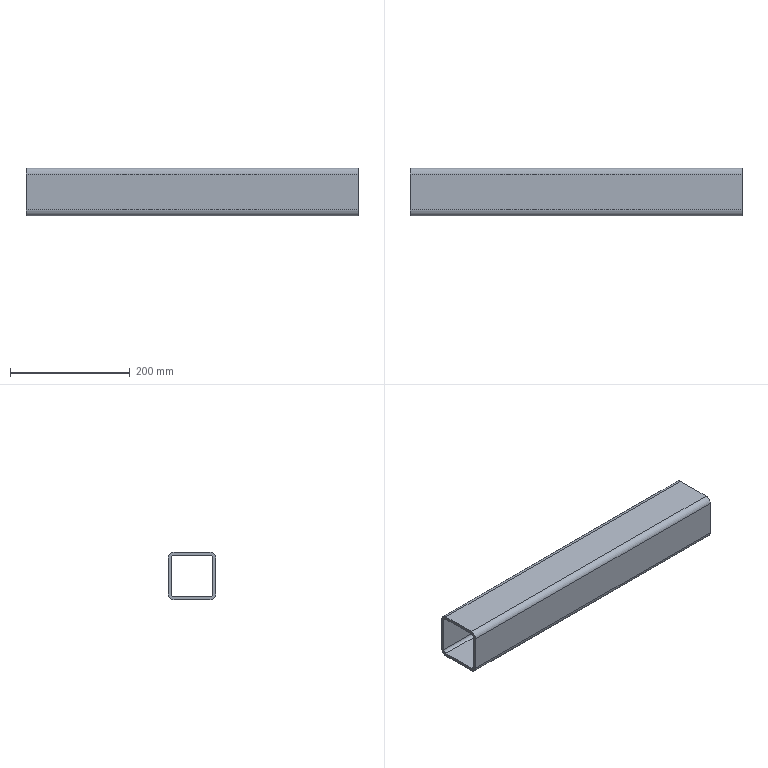Part | SolidWorks | features BaseBody 1 | 1 solid | 18 faces | box 555 x 80 x 80 mm | volume 796769 mm3 | plane 10 | cylinder 8 | commonest cylinder face diameters 10 x4 20 x4
STEP:
#1=CARTESIAN_POINT('',(-277.5,30.,-40.));
#2=VERTEX_POINT('',#1);
#3=CARTESIAN_POINT('',(-277.5,40.,-30.));
#4=VERTEX_POINT('',#3);
#5=CARTESIAN_POINT('',(-277.5,30.,-30.));
#6=DIRECTION('',(1.,0.,0.));
#7=DIRECTION('',(0.,0.,-1.));
#8=AXIS2_PLACEMENT_3D('',#5,#6,#7);
#9=CIRCLE('',#8,10.);
#10=EDGE_CURVE('',#2,#4,#9,.T.);
#11=ORIENTED_EDGE('',*,*,#10,.T.);
#12=CARTESIAN_POINT('',(277.5,40.,-30.));
#13=VERTEX_POINT('',#12);
#14=CARTESIAN_POINT('',(277.5,40.,-30.));
#15=DIRECTION('',(-1.,0.,0.));
#16=VECTOR('',#15,1000.);
#17=LINE('',#14,#16);
#18=EDGE_CURVE('',#13,#4,#17,.T.);
#19=ORIENTED_EDGE('',*,*,#18,.F.);
#20=CARTESIAN_POINT('',(277.5,30.,-40.));
#21=VERTEX_POINT('',#20);
#22=CARTESIAN_POINT('',(277.5,30.,-30.));
#23=DIRECTION('',(1.,0.,0.));
#24=DIRECTION('',(0.,0.,-1.));
#25=AXIS2_PLACEMENT_3D('',#22,#23,#24);
#26=CIRCLE('',#25,10.);
#27=EDGE_CURVE('',#21,#13,#26,.T.);
#28=ORIENTED_EDGE('',*,*,#27,.F.);
#29=CARTESIAN_POINT('',(277.5,30.,-40.));
#30=DIRECTION('',(-1.,0.,0.));
#31=VECTOR('',#30,1000.);
#32=LINE('',#29,#31);
#33=EDGE_CURVE('',#21,#2,#32,.T.);
#34=ORIENTED_EDGE('',*,*,#33,.T.);
#35=EDGE_LOOP('',(#11,#19,#28,#34));
#36=FACE_OUTER_BOUND('',#35,.T.);
#37=CARTESIAN_POINT('',(277.5,30.,-30.));
#38=DIRECTION('',(-1.,0.,0.));
#39=DIRECTION('',(0.,0.,1.));
#40=AXIS2_PLACEMENT_3D('',#37,#38,#39);
#41=CYLINDRICAL_SURFACE('',#40,10.);
#42=ADVANCED_FACE('',(#36),#41,.T.);
#43=CARTESIAN_POINT('',(-277.5,40.,30.));
#44=VERTEX_POINT('',#43);
#45=CARTESIAN_POINT('',(-277.5,40.,-30.));
#46=DIRECTION('',(0.,0.,1.));
#47=VECTOR('',#46,1000.);
#48=LINE('',#45,#47);
#49=EDGE_CURVE('',#4,#44,#48,.T.);
#50=ORIENTED_EDGE('',*,*,#49,.T.);
#51=CARTESIAN_POINT('',(277.5,40.,30.));
#52=VERTEX_POINT('',#51);
#53=CARTESIAN_POINT('',(277.5,40.,30.));
#54=DIRECTION('',(-1.,0.,0.));
#55=VECTOR('',#54,1000.);
#56=LINE('',#53,#55);
#57=EDGE_CURVE('',#52,#44,#56,.T.);
#58=ORIENTED_EDGE('',*,*,#57,.F.);
#59=CARTESIAN_POINT('',(277.5,40.,-30.));
#60=DIRECTION('',(0.,0.,1.));
#61=VECTOR('',#60,1000.);
#62=LINE('',#59,#61);
#63=EDGE_CURVE('',#13,#52,#62,.T.);
#64=ORIENTED_EDGE('',*,*,#63,.F.);
#65=ORIENTED_EDGE('',*,*,#18,.T.);
#66=EDGE_LOOP('',(#50,#58,#64,#65));
#67=FACE_OUTER_BOUND('',#66,.T.);
#68=CARTESIAN_POINT('',(277.5,40.,-30.));
#69=DIRECTION('',(0.,-1.,0.));
#70=DIRECTION('',(0.,0.,-1.));
#71=AXIS2_PLACEMENT_3D('',#68,#69,#70);
#72=PLANE('',#71);
#73=ADVANCED_FACE('',(#67),#72,.F.);
#74=CARTESIAN_POINT('',(-277.5,30.,40.));
#75=VERTEX_POINT('',#74);
#76=CARTESIAN_POINT('',(-277.5,30.,30.));
#77=DIRECTION('',(1.,0.,0.));
#78=DIRECTION('',(0.,0.,-1.));
#79=AXIS2_PLACEMENT_3D('',#76,#77,#78);
#80=CIRCLE('',#79,10.);
#81=EDGE_CURVE('',#44,#75,#80,.T.);
#82=ORIENTED_EDGE('',*,*,#81,.T.);
#83=CARTESIAN_POINT('',(277.5,30.,40.));
#84=VERTEX_POINT('',#83);
#85=CARTESIAN_POINT('',(277.5,30.,40.));
#86=DIRECTION('',(-1.,0.,0.));
#87=VECTOR('',#86,1000.);
#88=LINE('',#85,#87);
#89=EDGE_CURVE('',#84,#75,#88,.T.);
#90=ORIENTED_EDGE('',*,*,#89,.F.);
#91=CARTESIAN_POINT('',(277.5,30.,30.));
#92=DIRECTION('',(1.,0.,0.));
#93=DIRECTION('',(0.,0.,-1.));
#94=AXIS2_PLACEMENT_3D('',#91,#92,#93);
#95=CIRCLE('',#94,10.);
#96=EDGE_CURVE('',#52,#84,#95,.T.);
#97=ORIENTED_EDGE('',*,*,#96,.F.);
#98=ORIENTED_EDGE('',*,*,#57,.T.);
#99=EDGE_LOOP('',(#82,#90,#97,#98));
#100=FACE_OUTER_BOUND('',#99,.T.);
#101=CARTESIAN_POINT('',(277.5,30.,30.));
#102=DIRECTION('',(-1.,0.,0.));
#103=DIRECTION('',(0.,0.,1.));
#104=AXIS2_PLACEMENT_3D('',#101,#102,#103);
#105=CYLINDRICAL_SURFACE('',#104,10.);
#106=ADVANCED_FACE('',(#100),#105,.T.);
#107=CARTESIAN_POINT('',(-277.5,-30.,40.));
#108=VERTEX_POINT('',#107);
#109=CARTESIAN_POINT('',(-277.5,-30.,40.));
#110=DIRECTION('',(0.,-1.,0.));
#111=VECTOR('',#110,1000.);
#112=LINE('',#109,#111);
#113=EDGE_CURVE('',#75,#108,#112,.T.);
#114=ORIENTED_EDGE('',*,*,#113,.T.);
#115=CARTESIAN_POINT('',(277.5,-30.,40.));
#116=VERTEX_POINT('',#115);
#117=CARTESIAN_POINT('',(277.5,-30.,40.));
#118=DIRECTION('',(-1.,0.,0.));
#119=VECTOR('',#118,1000.);
#120=LINE('',#117,#119);
#121=EDGE_CURVE('',#116,#108,#120,.T.);
#122=ORIENTED_EDGE('',*,*,#121,.F.);
#123=CARTESIAN_POINT('',(277.5,-30.,40.));
#124=DIRECTION('',(0.,-1.,0.));
#125=VECTOR('',#124,1000.);
#126=LINE('',#123,#125);
#127=EDGE_CURVE('',#84,#116,#126,.T.);
#128=ORIENTED_EDGE('',*,*,#127,.F.);
#129=ORIENTED_EDGE('',*,*,#89,.T.);
#130=EDGE_LOOP('',(#114,#122,#128,#129));
#131=FACE_OUTER_BOUND('',#130,.T.);
#132=CARTESIAN_POINT('',(277.5,-30.,40.));
#133=DIRECTION('',(0.,0.,-1.));
#134=DIRECTION('',(-1.,0.,0.));
#135=AXIS2_PLACEMENT_3D('',#132,#133,#134);
#136=PLANE('',#135);
#137=ADVANCED_FACE('',(#131),#136,.F.);
#138=CARTESIAN_POINT('',(-277.5,-40.,30.));
#139=VERTEX_POINT('',#138);
#140=CARTESIAN_POINT('',(-277.5,-30.,30.));
#141=DIRECTION('',(1.,0.,0.));
#142=DIRECTION('',(0.,0.,-1.));
#143=AXIS2_PLACEMENT_3D('',#140,#141,#142);
#144=CIRCLE('',#143,10.);
#145=EDGE_CURVE('',#108,#139,#144,.T.);
#146=ORIENTED_EDGE('',*,*,#145,.T.);
#147=CARTESIAN_POINT('',(277.5,-40.,30.));
#148=VERTEX_POINT('',#147);
#149=CARTESIAN_POINT('',(277.5,-40.,30.));
#150=DIRECTION('',(-1.,0.,0.));
#151=VECTOR('',#150,1000.);
#152=LINE('',#149,#151);
#153=EDGE_CURVE('',#148,#139,#152,.T.);
#154=ORIENTED_EDGE('',*,*,#153,.F.);
#155=CARTESIAN_POINT('',(277.5,-30.,30.));
#156=DIRECTION('',(1.,0.,0.));
#157=DIRECTION('',(0.,0.,-1.));
#158=AXIS2_PLACEMENT_3D('',#155,#156,#157);
#159=CIRCLE('',#158,10.);
#160=EDGE_CURVE('',#116,#148,#159,.T.);
#161=ORIENTED_EDGE('',*,*,#160,.F.);
#162=ORIENTED_EDGE('',*,*,#121,.T.);
#163=EDGE_LOOP('',(#146,#154,#161,#162));
#164=FACE_OUTER_BOUND('',#163,.T.);
#165=CARTESIAN_POINT('',(277.5,-30.,30.));
#166=DIRECTION('',(-1.,0.,0.));
#167=DIRECTION('',(0.,0.,1.));
#168=AXIS2_PLACEMENT_3D('',#165,#166,#167);
#169=CYLINDRICAL_SURFACE('',#168,10.);
#170=ADVANCED_FACE('',(#164),#169,.T.);
#171=CARTESIAN_POINT('',(-277.5,-40.,-30.));
#172=VERTEX_POINT('',#171);
#173=CARTESIAN_POINT('',(-277.5,-40.,30.));
#174=DIRECTION('',(0.,0.,-1.));
#175=VECTOR('',#174,1000.);
#176=LINE('',#173,#175);
#177=EDGE_CURVE('',#139,#172,#176,.T.);
#178=ORIENTED_EDGE('',*,*,#177,.T.);
#179=CARTESIAN_POINT('',(277.5,-40.,-30.));
#180=VERTEX_POINT('',#179);
#181=CARTESIAN_POINT('',(277.5,-40.,-30.));
#182=DIRECTION('',(-1.,0.,0.));
#183=VECTOR('',#182,1000.);
#184=LINE('',#181,#183);
#185=EDGE_CURVE('',#180,#172,#184,.T.);
#186=ORIENTED_EDGE('',*,*,#185,.F.);
#187=CARTESIAN_POINT('',(277.5,-40.,30.));
#188=DIRECTION('',(0.,0.,-1.));
#189=VECTOR('',#188,1000.);
#190=LINE('',#187,#189);
#191=EDGE_CURVE('',#148,#180,#190,.T.);
#192=ORIENTED_EDGE('',*,*,#191,.F.);
#193=ORIENTED_EDGE('',*,*,#153,.T.);
#194=EDGE_LOOP('',(#178,#186,#192,#193));
#195=FACE_OUTER_BOUND('',#194,.T.);
#196=CARTESIAN_POINT('',(277.5,-40.,30.));
#197=DIRECTION('',(0.,1.,0.));
#198=DIRECTION('',(0.,0.,1.));
#199=AXIS2_PLACEMENT_3D('',#196,#197,#198);
#200=PLANE('',#199);
#201=ADVANCED_FACE('',(#195),#200,.F.);
#202=CARTESIAN_POINT('',(-277.5,-30.,-40.));
#203=VERTEX_POINT('',#202);
#204=CARTESIAN_POINT('',(-277.5,-30.,-30.));
#205=DIRECTION('',(1.,0.,0.));
#206=DIRECTION('',(0.,0.,-1.));
#207=AXIS2_PLACEMENT_3D('',#204,#205,#206);
#208=CIRCLE('',#207,10.);
#209=EDGE_CURVE('',#172,#203,#208,.T.);
#210=ORIENTED_EDGE('',*,*,#209,.T.);
#211=CARTESIAN_POINT('',(277.5,-30.,-40.));
#212=VERTEX_POINT('',#211);
#213=CARTESIAN_POINT('',(277.5,-30.,-40.));
#214=DIRECTION('',(-1.,0.,0.));
#215=VECTOR('',#214,1000.);
#216=LINE('',#213,#215);
#217=EDGE_CURVE('',#212,#203,#216,.T.);
#218=ORIENTED_EDGE('',*,*,#217,.F.);
#219=CARTESIAN_POINT('',(277.5,-30.,-30.));
#220=DIRECTION('',(1.,0.,0.));
#221=DIRECTION('',(0.,0.,-1.));
#222=AXIS2_PLACEMENT_3D('',#219,#220,#221);
#223=CIRCLE('',#222,10.);
#224=EDGE_CURVE('',#180,#212,#223,.T.);
#225=ORIENTED_EDGE('',*,*,#224,.F.);
#226=ORIENTED_EDGE('',*,*,#185,.T.);
#227=EDGE_LOOP('',(#210,#218,#225,#226));
#228=FACE_OUTER_BOUND('',#227,.T.);
#229=CARTESIAN_POINT('',(277.5,-30.,-30.));
#230=DIRECTION('',(-1.,0.,0.));
#231=DIRECTION('',(0.,0.,1.));
#232=AXIS2_PLACEMENT_3D('',#229,#230,#231);
#233=CYLINDRICAL_SURFACE('',#232,10.);
#234=ADVANCED_FACE('',(#228),#233,.T.);
#235=CARTESIAN_POINT('',(-277.5,35.,30.));
#236=VERTEX_POINT('',#235);
#237=CARTESIAN_POINT('',(-277.5,30.,35.));
#238=VERTEX_POINT('',#237);
#239=CARTESIAN_POINT('',(-277.5,30.,30.));
#240=DIRECTION('',(1.,0.,0.));
#241=DIRECTION('',(0.,0.,-1.));
#242=AXIS2_PLACEMENT_3D('',#239,#240,#241);
#243=CIRCLE('',#242,5.);
#244=EDGE_CURVE('',#236,#238,#243,.T.);
#245=ORIENTED_EDGE('',*,*,#244,.F.);
#246=CARTESIAN_POINT('',(277.5,35.,30.));
#247=VERTEX_POINT('',#246);
#248=CARTESIAN_POINT('',(277.5,35.,30.));
#249=DIRECTION('',(-1.,0.,0.));
#250=VECTOR('',#249,1000.);
#251=LINE('',#248,#250);
#252=EDGE_CURVE('',#247,#236,#251,.T.);
#253=ORIENTED_EDGE('',*,*,#252,.F.);
#254=CARTESIAN_POINT('',(277.5,30.,35.));
#255=VERTEX_POINT('',#254);
#256=CARTESIAN_POINT('',(277.5,30.,30.));
#257=DIRECTION('',(1.,0.,0.));
#258=DIRECTION('',(0.,0.,-1.));
#259=AXIS2_PLACEMENT_3D('',#256,#257,#258);
#260=CIRCLE('',#259,5.);
#261=EDGE_CURVE('',#247,#255,#260,.T.);
#262=ORIENTED_EDGE('',*,*,#261,.T.);
#263=CARTESIAN_POINT('',(277.5,30.,35.));
#264=DIRECTION('',(-1.,0.,0.));
#265=VECTOR('',#264,1000.);
#266=LINE('',#263,#265);
#267=EDGE_CURVE('',#255,#238,#266,.T.);
#268=ORIENTED_EDGE('',*,*,#267,.T.);
#269=EDGE_LOOP('',(#245,#253,#262,#268));
#270=FACE_OUTER_BOUND('',#269,.T.);
#271=CARTESIAN_POINT('',(277.5,30.,30.));
#272=DIRECTION('',(-1.,0.,0.));
#273=DIRECTION('',(0.,0.,1.));
#274=AXIS2_PLACEMENT_3D('',#271,#272,#273);
#275=CYLINDRICAL_SURFACE('',#274,5.);
#276=ADVANCED_FACE('',(#270),#275,.F.);
#277=CARTESIAN_POINT('',(-277.5,35.,-30.));
#278=VERTEX_POINT('',#277);
#279=CARTESIAN_POINT('',(-277.5,35.,-30.));
#280=DIRECTION('',(0.,0.,1.));
#281=VECTOR('',#280,1000.);
#282=LINE('',#279,#281);
#283=EDGE_CURVE('',#278,#236,#282,.T.);
#284=ORIENTED_EDGE('',*,*,#283,.F.);
#285=CARTESIAN_POINT('',(277.5,35.,-30.));
#286=VERTEX_POINT('',#285);
#287=CARTESIAN_POINT('',(277.5,35.,-30.));
#288=DIRECTION('',(-1.,0.,0.));
#289=VECTOR('',#288,1000.);
#290=LINE('',#287,#289);
#291=EDGE_CURVE('',#286,#278,#290,.T.);
#292=ORIENTED_EDGE('',*,*,#291,.F.);
#293=CARTESIAN_POINT('',(277.5,35.,-30.));
#294=DIRECTION('',(0.,0.,1.));
#295=VECTOR('',#294,1000.);
#296=LINE('',#293,#295);
#297=EDGE_CURVE('',#286,#247,#296,.T.);
#298=ORIENTED_EDGE('',*,*,#297,.T.);
#299=ORIENTED_EDGE('',*,*,#252,.T.);
#300=EDGE_LOOP('',(#284,#292,#298,#299));
#301=FACE_OUTER_BOUND('',#300,.T.);
#302=CARTESIAN_POINT('',(277.5,35.,-30.));
#303=DIRECTION('',(0.,-1.,0.));
#304=DIRECTION('',(0.,0.,-1.));
#305=AXIS2_PLACEMENT_3D('',#302,#303,#304);
#306=PLANE('',#305);
#307=ADVANCED_FACE('',(#301),#306,.T.);
#308=CARTESIAN_POINT('',(-277.5,30.,-35.));
#309=VERTEX_POINT('',#308);
#310=CARTESIAN_POINT('',(-277.5,30.,-30.));
#311=DIRECTION('',(1.,0.,0.));
#312=DIRECTION('',(0.,0.,-1.));
#313=AXIS2_PLACEMENT_3D('',#310,#311,#312);
#314=CIRCLE('',#313,5.);
#315=EDGE_CURVE('',#309,#278,#314,.T.);
#316=ORIENTED_EDGE('',*,*,#315,.F.);
#317=CARTESIAN_POINT('',(277.5,30.,-35.));
#318=VERTEX_POINT('',#317);
#319=CARTESIAN_POINT('',(277.5,30.,-35.));
#320=DIRECTION('',(-1.,0.,0.));
#321=VECTOR('',#320,1000.);
#322=LINE('',#319,#321);
#323=EDGE_CURVE('',#318,#309,#322,.T.);
#324=ORIENTED_EDGE('',*,*,#323,.F.);
#325=CARTESIAN_POINT('',(277.5,30.,-30.));
#326=DIRECTION('',(1.,0.,0.));
#327=DIRECTION('',(0.,0.,-1.));
#328=AXIS2_PLACEMENT_3D('',#325,#326,#327);
#329=CIRCLE('',#328,5.);
#330=EDGE_CURVE('',#318,#286,#329,.T.);
#331=ORIENTED_EDGE('',*,*,#330,.T.);
#332=ORIENTED_EDGE('',*,*,#291,.T.);
#333=EDGE_LOOP('',(#316,#324,#331,#332));
#334=FACE_OUTER_BOUND('',#333,.T.);
#335=CARTESIAN_POINT('',(277.5,30.,-30.));
#336=DIRECTION('',(-1.,0.,0.));
#337=DIRECTION('',(0.,0.,1.));
#338=AXIS2_PLACEMENT_3D('',#335,#336,#337);
#339=CYLINDRICAL_SURFACE('',#338,5.);
#340=ADVANCED_FACE('',(#334),#339,.F.);
#341=CARTESIAN_POINT('',(-277.5,-30.,-35.));
#342=VERTEX_POINT('',#341);
#343=CARTESIAN_POINT('',(-277.5,30.,-35.));
#344=DIRECTION('',(0.,1.,0.));
#345=VECTOR('',#344,1000.);
#346=LINE('',#343,#345);
#347=EDGE_CURVE('',#342,#309,#346,.T.);
#348=ORIENTED_EDGE('',*,*,#347,.F.);
#349=CARTESIAN_POINT('',(277.5,-30.,-35.));
#350=VERTEX_POINT('',#349);
#351=CARTESIAN_POINT('',(277.5,-30.,-35.));
#352=DIRECTION('',(-1.,0.,0.));
#353=VECTOR('',#352,1000.);
#354=LINE('',#351,#353);
#355=EDGE_CURVE('',#350,#342,#354,.T.);
#356=ORIENTED_EDGE('',*,*,#355,.F.);
#357=CARTESIAN_POINT('',(277.5,30.,-35.));
#358=DIRECTION('',(0.,1.,0.));
#359=VECTOR('',#358,1000.);
#360=LINE('',#357,#359);
#361=EDGE_CURVE('',#350,#318,#360,.T.);
#362=ORIENTED_EDGE('',*,*,#361,.T.);
#363=ORIENTED_EDGE('',*,*,#323,.T.);
#364=EDGE_LOOP('',(#348,#356,#362,#363));
#365=FACE_OUTER_BOUND('',#364,.T.);
#366=CARTESIAN_POINT('',(277.5,30.,-35.));
#367=DIRECTION('',(0.,0.,1.));
#368=DIRECTION('',(1.,0.,0.));
#369=AXIS2_PLACEMENT_3D('',#366,#367,#368);
#370=PLANE('',#369);
#371=ADVANCED_FACE('',(#365),#370,.T.);
#372=CARTESIAN_POINT('',(-277.5,-35.,-30.));
#373=VERTEX_POINT('',#372);
#374=CARTESIAN_POINT('',(-277.5,-30.,-30.));
#375=DIRECTION('',(1.,0.,0.));
#376=DIRECTION('',(0.,0.,-1.));
#377=AXIS2_PLACEMENT_3D('',#374,#375,#376);
#378=CIRCLE('',#377,5.);
#379=EDGE_CURVE('',#373,#342,#378,.T.);
#380=ORIENTED_EDGE('',*,*,#379,.F.);
#381=CARTESIAN_POINT('',(277.5,-35.,-30.));
#382=VERTEX_POINT('',#381);
#383=CARTESIAN_POINT('',(277.5,-35.,-30.));
#384=DIRECTION('',(-1.,0.,0.));
#385=VECTOR('',#384,1000.);
#386=LINE('',#383,#385);
#387=EDGE_CURVE('',#382,#373,#386,.T.);
#388=ORIENTED_EDGE('',*,*,#387,.F.);
#389=CARTESIAN_POINT('',(277.5,-30.,-30.));
#390=DIRECTION('',(1.,0.,0.));
#391=DIRECTION('',(0.,0.,-1.));
#392=AXIS2_PLACEMENT_3D('',#389,#390,#391);
#393=CIRCLE('',#392,5.);
#394=EDGE_CURVE('',#382,#350,#393,.T.);
#395=ORIENTED_EDGE('',*,*,#394,.T.);
#396=ORIENTED_EDGE('',*,*,#355,.T.);
#397=EDGE_LOOP('',(#380,#388,#395,#396));
#398=FACE_OUTER_BOUND('',#397,.T.);
#399=CARTESIAN_POINT('',(277.5,-30.,-30.));
#400=DIRECTION('',(-1.,0.,0.));
#401=DIRECTION('',(0.,0.,1.));
#402=AXIS2_PLACEMENT_3D('',#399,#400,#401);
#403=CYLINDRICAL_SURFACE('',#402,5.);
#404=ADVANCED_FACE('',(#398),#403,.F.);
#405=CARTESIAN_POINT('',(-277.5,-35.,30.));
#406=VERTEX_POINT('',#405);
#407=CARTESIAN_POINT('',(-277.5,-35.,30.));
#408=DIRECTION('',(0.,0.,-1.));
#409=VECTOR('',#408,1000.);
#410=LINE('',#407,#409);
#411=EDGE_CURVE('',#406,#373,#410,.T.);
#412=ORIENTED_EDGE('',*,*,#411,.F.);
#413=CARTESIAN_POINT('',(277.5,-35.,30.));
#414=VERTEX_POINT('',#413);
#415=CARTESIAN_POINT('',(277.5,-35.,30.));
#416=DIRECTION('',(-1.,0.,0.));
#417=VECTOR('',#416,1000.);
#418=LINE('',#415,#417);
#419=EDGE_CURVE('',#414,#406,#418,.T.);
#420=ORIENTED_EDGE('',*,*,#419,.F.);
#421=CARTESIAN_POINT('',(277.5,-35.,30.));
#422=DIRECTION('',(0.,0.,-1.));
#423=VECTOR('',#422,1000.);
#424=LINE('',#421,#423);
#425=EDGE_CURVE('',#414,#382,#424,.T.);
#426=ORIENTED_EDGE('',*,*,#425,.T.);
#427=ORIENTED_EDGE('',*,*,#387,.T.);
#428=EDGE_LOOP('',(#412,#420,#426,#427));
#429=FACE_OUTER_BOUND('',#428,.T.);
#430=CARTESIAN_POINT('',(277.5,-35.,30.));
#431=DIRECTION('',(0.,1.,0.));
#432=DIRECTION('',(0.,0.,1.));
#433=AXIS2_PLACEMENT_3D('',#430,#431,#432);
#434=PLANE('',#433);
#435=ADVANCED_FACE('',(#429),#434,.T.);
#436=CARTESIAN_POINT('',(-277.5,-30.,35.));
#437=VERTEX_POINT('',#436);
#438=CARTESIAN_POINT('',(-277.5,-30.,30.));
#439=DIRECTION('',(1.,0.,0.));
#440=DIRECTION('',(0.,0.,-1.));
#441=AXIS2_PLACEMENT_3D('',#438,#439,#440);
#442=CIRCLE('',#441,5.);
#443=EDGE_CURVE('',#437,#406,#442,.T.);
#444=ORIENTED_EDGE('',*,*,#443,.F.);
#445=CARTESIAN_POINT('',(277.5,-30.,35.));
#446=VERTEX_POINT('',#445);
#447=CARTESIAN_POINT('',(277.5,-30.,35.));
#448=DIRECTION('',(-1.,0.,0.));
#449=VECTOR('',#448,1000.);
#450=LINE('',#447,#449);
#451=EDGE_CURVE('',#446,#437,#450,.T.);
#452=ORIENTED_EDGE('',*,*,#451,.F.);
#453=CARTESIAN_POINT('',(277.5,-30.,30.));
#454=DIRECTION('',(1.,0.,0.));
#455=DIRECTION('',(0.,0.,-1.));
#456=AXIS2_PLACEMENT_3D('',#453,#454,#455);
#457=CIRCLE('',#456,5.);
#458=EDGE_CURVE('',#446,#414,#457,.T.);
#459=ORIENTED_EDGE('',*,*,#458,.T.);
#460=ORIENTED_EDGE('',*,*,#419,.T.);
#461=EDGE_LOOP('',(#444,#452,#459,#460));
#462=FACE_OUTER_BOUND('',#461,.T.);
#463=CARTESIAN_POINT('',(277.5,-30.,30.));
#464=DIRECTION('',(-1.,0.,0.));
#465=DIRECTION('',(0.,0.,1.));
#466=AXIS2_PLACEMENT_3D('',#463,#464,#465);
#467=CYLINDRICAL_SURFACE('',#466,5.);
#468=ADVANCED_FACE('',(#462),#467,.F.);
#469=CARTESIAN_POINT('',(-277.5,-30.,35.));
#470=DIRECTION('',(0.,-1.,0.));
#471=VECTOR('',#470,1000.);
#472=LINE('',#469,#471);
#473=EDGE_CURVE('',#238,#437,#472,.T.);
#474=ORIENTED_EDGE('',*,*,#473,.F.);
#475=ORIENTED_EDGE('',*,*,#267,.F.);
#476=CARTESIAN_POINT('',(277.5,-30.,35.));
#477=DIRECTION('',(0.,-1.,0.));
#478=VECTOR('',#477,1000.);
#479=LINE('',#476,#478);
#480=EDGE_CURVE('',#255,#446,#479,.T.);
#481=ORIENTED_EDGE('',*,*,#480,.T.);
#482=ORIENTED_EDGE('',*,*,#451,.T.);
#483=EDGE_LOOP('',(#474,#475,#481,#482));
#484=FACE_OUTER_BOUND('',#483,.T.);
#485=CARTESIAN_POINT('',(277.5,-30.,35.));
#486=DIRECTION('',(0.,0.,-1.));
#487=DIRECTION('',(-1.,0.,0.));
#488=AXIS2_PLACEMENT_3D('',#485,#486,#487);
#489=PLANE('',#488);
#490=ADVANCED_FACE('',(#484),#489,.T.);
#491=CARTESIAN_POINT('',(-277.5,30.,-40.));
#492=DIRECTION('',(0.,1.,0.));
#493=VECTOR('',#492,1000.);
#494=LINE('',#491,#493);
#495=EDGE_CURVE('',#203,#2,#494,.T.);
#496=ORIENTED_EDGE('',*,*,#495,.T.);
#497=ORIENTED_EDGE('',*,*,#33,.F.);
#498=CARTESIAN_POINT('',(277.5,30.,-40.));
#499=DIRECTION('',(0.,1.,0.));
#500=VECTOR('',#499,1000.);
#501=LINE('',#498,#500);
#502=EDGE_CURVE('',#212,#21,#501,.T.);
#503=ORIENTED_EDGE('',*,*,#502,.F.);
#504=ORIENTED_EDGE('',*,*,#217,.T.);
#505=EDGE_LOOP('',(#496,#497,#503,#504));
#506=FACE_OUTER_BOUND('',#505,.T.);
#507=CARTESIAN_POINT('',(277.5,30.,-40.));
#508=DIRECTION('',(0.,0.,1.));
#509=DIRECTION('',(1.,0.,0.));
#510=AXIS2_PLACEMENT_3D('',#507,#508,#509);
#511=PLANE('',#510);
#512=ADVANCED_FACE('',(#506),#511,.F.);
#513=ORIENTED_EDGE('',*,*,#261,.F.);
#514=ORIENTED_EDGE('',*,*,#297,.F.);
#515=ORIENTED_EDGE('',*,*,#330,.F.);
#516=ORIENTED_EDGE('',*,*,#361,.F.);
#517=ORIENTED_EDGE('',*,*,#394,.F.);
#518=ORIENTED_EDGE('',*,*,#425,.F.);
#519=ORIENTED_EDGE('',*,*,#458,.F.);
#520=ORIENTED_EDGE('',*,*,#480,.F.);
#521=EDGE_LOOP('',(#513,#514,#515,#516,#517,#518,#519,#520));
#522=FACE_BOUND('',#521,.T.);
#523=ORIENTED_EDGE('',*,*,#27,.T.);
#524=ORIENTED_EDGE('',*,*,#63,.T.);
#525=ORIENTED_EDGE('',*,*,#96,.T.);
#526=ORIENTED_EDGE('',*,*,#127,.T.);
#527=ORIENTED_EDGE('',*,*,#160,.T.);
#528=ORIENTED_EDGE('',*,*,#191,.T.);
#529=ORIENTED_EDGE('',*,*,#224,.T.);
#530=ORIENTED_EDGE('',*,*,#502,.T.);
#531=EDGE_LOOP('',(#523,#524,#525,#526,#527,#528,#529,#530));
#532=FACE_OUTER_BOUND('',#531,.T.);
#533=CARTESIAN_POINT('',(277.5,30.,-30.));
#534=DIRECTION('',(1.,0.,0.));
#535=DIRECTION('',(0.,0.,-1.));
#536=AXIS2_PLACEMENT_3D('',#533,#534,#535);
#537=PLANE('',#536);
#538=ADVANCED_FACE('',(#522,#532),#537,.T.);
#539=ORIENTED_EDGE('',*,*,#244,.T.);
#540=ORIENTED_EDGE('',*,*,#473,.T.);
#541=ORIENTED_EDGE('',*,*,#443,.T.);
#542=ORIENTED_EDGE('',*,*,#411,.T.);
#543=ORIENTED_EDGE('',*,*,#379,.T.);
#544=ORIENTED_EDGE('',*,*,#347,.T.);
#545=ORIENTED_EDGE('',*,*,#315,.T.);
#546=ORIENTED_EDGE('',*,*,#283,.T.);
#547=EDGE_LOOP('',(#539,#540,#541,#542,#543,#544,#545,#546));
#548=FACE_BOUND('',#547,.T.);
#549=ORIENTED_EDGE('',*,*,#10,.F.);
#550=ORIENTED_EDGE('',*,*,#495,.F.);
#551=ORIENTED_EDGE('',*,*,#209,.F.);
#552=ORIENTED_EDGE('',*,*,#177,.F.);
#553=ORIENTED_EDGE('',*,*,#145,.F.);
#554=ORIENTED_EDGE('',*,*,#113,.F.);
#555=ORIENTED_EDGE('',*,*,#81,.F.);
#556=ORIENTED_EDGE('',*,*,#49,.F.);
#557=EDGE_LOOP('',(#549,#550,#551,#552,#553,#554,#555,#556));
#558=FACE_OUTER_BOUND('',#557,.T.);
#559=CARTESIAN_POINT('',(-277.5,30.,-30.));
#560=DIRECTION('',(1.,0.,0.));
#561=DIRECTION('',(0.,0.,-1.));
#562=AXIS2_PLACEMENT_3D('',#559,#560,#561);
#563=PLANE('',#562);
#564=ADVANCED_FACE('',(#548,#558),#563,.F.);
#565=CLOSED_SHELL('',(#42,#73,#106,#137,#170,#201,#234,#276,#307,#340,#371,#404,#435,#468,#490,#512,#538,#564));
#566=MANIFOLD_SOLID_BREP('',#565);
#567=CARTESIAN_POINT('',(0.,0.,0.));
#568=DIRECTION('',(0.,0.,1.));
#569=DIRECTION('',(1.,0.,0.));
#570=AXIS2_PLACEMENT_3D('',#567,#568,#569);
#571=(LENGTH_UNIT()NAMED_UNIT(*)SI_UNIT(.MILLI.,.METRE.));
#572=UNCERTAINTY_MEASURE_WITH_UNIT(LENGTH_MEASURE(0.00001),#571,'','');
#573=(NAMED_UNIT(*)PLANE_ANGLE_UNIT()SI_UNIT($,.RADIAN.));
#574=(NAMED_UNIT(*)SI_UNIT($,.STERADIAN.)SOLID_ANGLE_UNIT());
#575=(GEOMETRIC_REPRESENTATION_CONTEXT(3)GLOBAL_UNCERTAINTY_ASSIGNED_CONTEXT((#572))GLOBAL_UNIT_ASSIGNED_CONTEXT((#571,#573,#574))REPRESENTATION_CONTEXT('',''));
#576=ADVANCED_BREP_SHAPE_REPRESENTATION('',(#566,#570),#575);